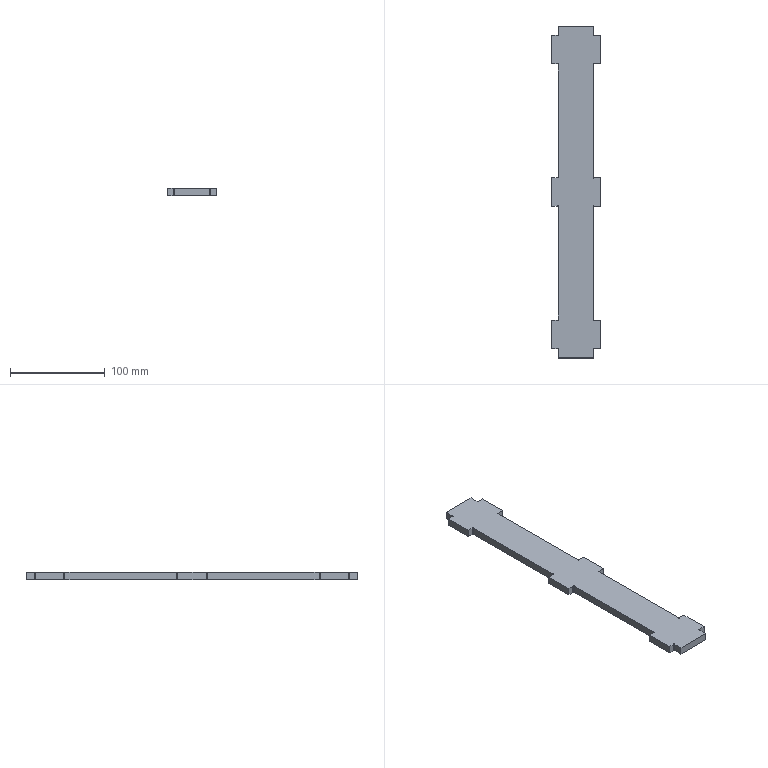Part | SolidWorks | features Fillet 1, FlatPattern 1, ICE 1, SMBaseFlange 1, SheetMetal 1 | 1 solid | 72 faces | box 51.5 x 350 x 8 mm | volume 114010 mm3 | cylinder 42 | plane 30 | commonest cylinder face diameters 2 x24 1 x18